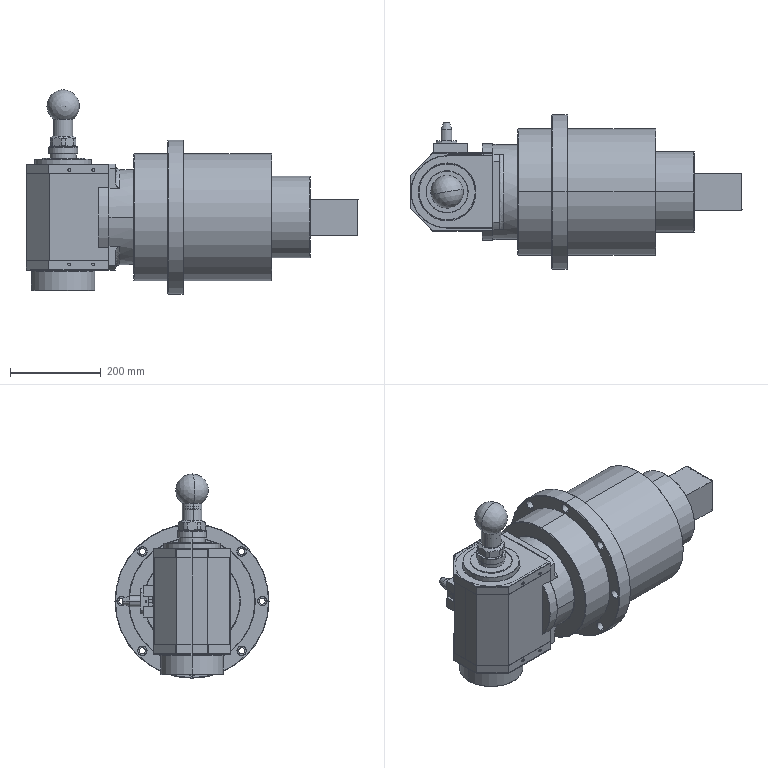Part | SolidWorks | 16 solids | 887 faces | box 732.6 x 340 x 450.98 mm | volume 29819658 mm3 | cylinder 359 | plane 301 | cone 221 | spline 4 | sphere 2 | commonest cylinder face diameters 5 x50 6.5 x32 9 x28 20 x22 5.5 x17 13 x16